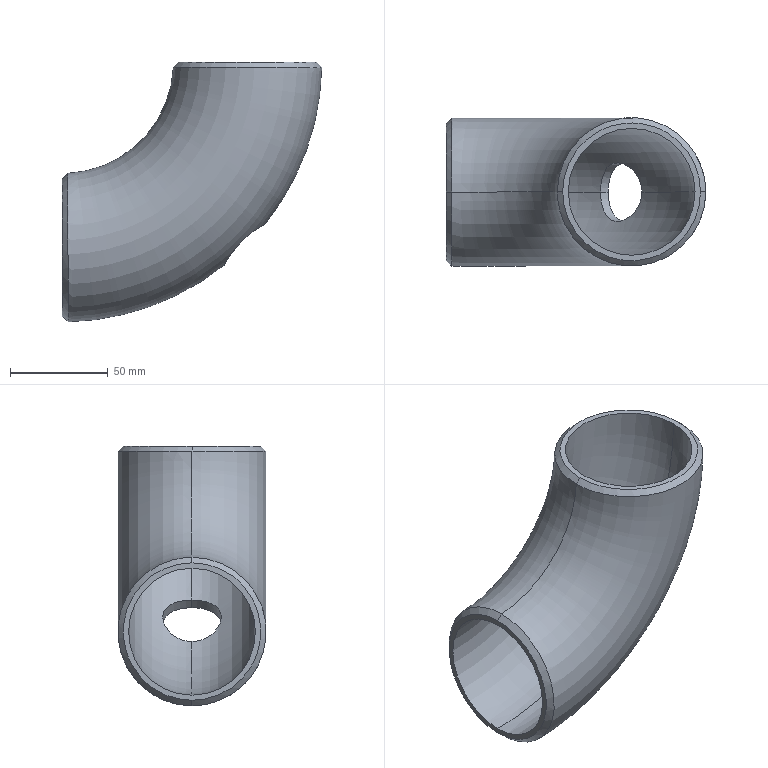Part | SolidWorks | features Chamfer 1, ICE 1, Revolution 1 | 1 solid | 12 faces | box 132.972 x 76 x 132.966 mm | volume 175775 mm3 | spline 4 | torus 4 | cylinder 2 | plane 2 | commonest cylinder face diameters 30 x2